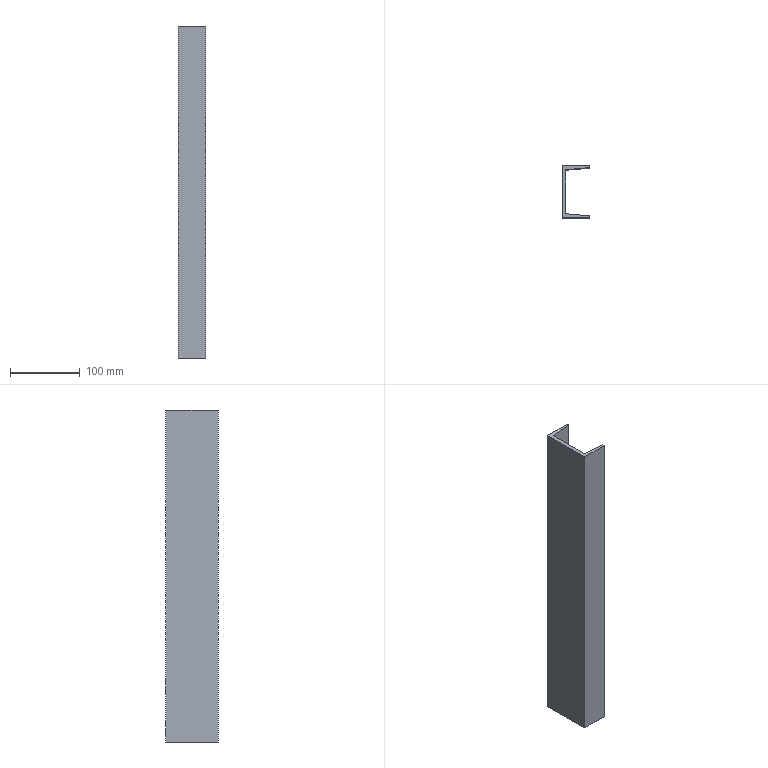Part | STEP file | BCC3 H13_8B | 1 solid | 20 faces | box 40 x 75 x 475 mm | volume 326568 mm3 | plane 14 | cylinder 6 | commonest cylinder face diameters 12 x6